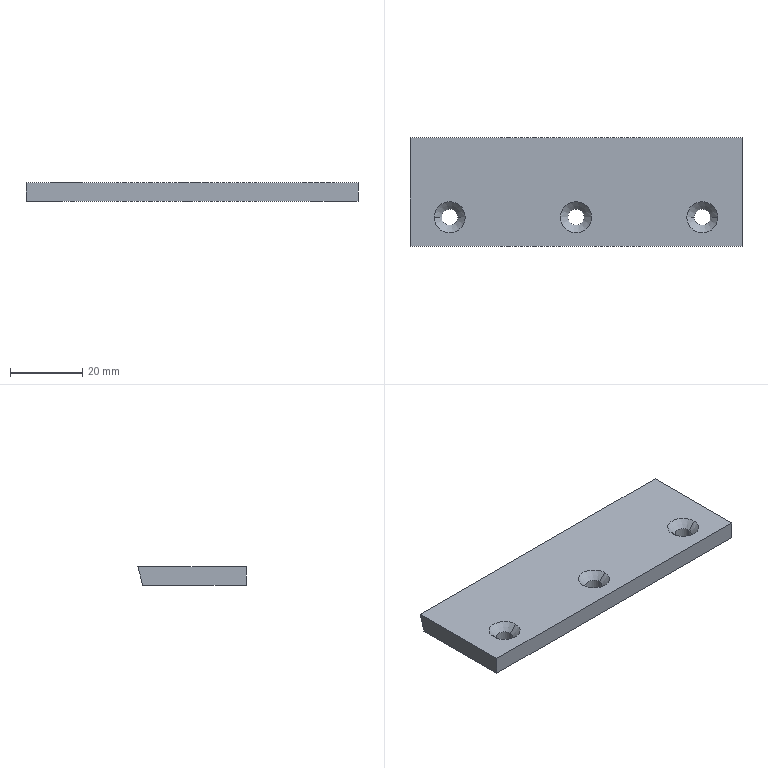Part | STEP file | 2030 Blade A | 1 solid | 18 faces | box 92 x 30 x 5 mm | volume 13137 mm3 | cone 6 | cylinder 6 | plane 6 | commonest cylinder face diameters 4.5 x6
STEP:
#1=CARTESIAN_POINT('',(0.,0.,0.));
#2=DIRECTION('',(0.,0.,1.));
#3=DIRECTION('',(1.,0.,0.));
#4=AXIS2_PLACEMENT_3D('',#1,#2,#3);
#5=CARTESIAN_POINT('',(-32.75,-7.,2.95));
#6=VERTEX_POINT('',#5);
#7=CARTESIAN_POINT('',(-30.7,-7.,5.));
#8=VERTEX_POINT('',#7);
#9=CARTESIAN_POINT('',(-30.7,-7.,5.));
#10=DIRECTION('',(0.7071,0.,0.7071));
#11=VECTOR('',#10,1.);
#12=LINE('',#9,#11);
#13=CARTESIAN_POINT('',(-35.,-7.,5.));
#14=DIRECTION('',(0.,0.,1.));
#15=DIRECTION('',(1.,0.,0.));
#16=AXIS2_PLACEMENT_3D('',#13,#14,#15);
#17=CONICAL_SURFACE('',#16,4.3,0.7854);
#18=CARTESIAN_POINT('',(6.283,0.));
#19=DIRECTION('',(0.,1.));
#20=VECTOR('',#19,1.);
#21=LINE('',#18,#20);
#22=(GEOMETRIC_REPRESENTATION_CONTEXT(2)PARAMETRIC_REPRESENTATION_CONTEXT()REPRESENTATION_CONTEXT('',''));
#23=DEFINITIONAL_REPRESENTATION('',(#21),#22);
#24=PCURVE('',#17,#23);
#25=CARTESIAN_POINT('',(-35.,-7.,5.));
#26=DIRECTION('',(0.,0.,1.));
#27=DIRECTION('',(1.,0.,0.));
#28=AXIS2_PLACEMENT_3D('',#25,#26,#27);
#29=CONICAL_SURFACE('',#28,4.3,0.7854);
#30=CARTESIAN_POINT('',(0.,0.));
#31=DIRECTION('',(0.,1.));
#32=VECTOR('',#31,1.);
#33=LINE('',#30,#32);
#34=(GEOMETRIC_REPRESENTATION_CONTEXT(2)PARAMETRIC_REPRESENTATION_CONTEXT()REPRESENTATION_CONTEXT('',''));
#35=DEFINITIONAL_REPRESENTATION('',(#33),#34);
#36=PCURVE('',#29,#35);
#37=SURFACE_CURVE('',#12,(#24,#36),.PCURVE_S1.);
#38=EDGE_CURVE('',#6,#8,#37,.T.);
#39=ORIENTED_EDGE('',*,*,#38,.T.);
#40=CARTESIAN_POINT('',(-39.3,-7.,5.));
#41=VERTEX_POINT('',#40);
#42=CARTESIAN_POINT('',(-35.,-7.,5.));
#43=DIRECTION('',(0.,0.,1.));
#44=DIRECTION('',(1.,0.,0.));
#45=AXIS2_PLACEMENT_3D('',#42,#43,#44);
#46=CIRCLE('',#45,4.3);
#47=CARTESIAN_POINT('',(0.,0.));
#48=DIRECTION('',(1.,0.));
#49=VECTOR('',#48,1.);
#50=LINE('',#47,#49);
#51=(GEOMETRIC_REPRESENTATION_CONTEXT(2)PARAMETRIC_REPRESENTATION_CONTEXT()REPRESENTATION_CONTEXT('',''));
#52=DEFINITIONAL_REPRESENTATION('',(#50),#51);
#53=PCURVE('',#17,#52);
#54=CARTESIAN_POINT('',(0.,0.,5.));
#55=DIRECTION('',(0.,0.,-1.));
#56=DIRECTION('',(-1.,0.,0.));
#57=AXIS2_PLACEMENT_3D('',#54,#55,#56);
#58=PLANE('',#57);
#59=CARTESIAN_POINT('',(30.7,-7.));
#60=CARTESIAN_POINT('',(30.7,0.4478));
#61=CARTESIAN_POINT('',(37.15,-3.276));
#62=CARTESIAN_POINT('',(43.6,-7.));
#63=CARTESIAN_POINT('',(37.15,-10.724));
#64=CARTESIAN_POINT('',(30.7,-14.448));
#65=CARTESIAN_POINT('',(30.7,-7.));
#66=(BOUNDED_CURVE()B_SPLINE_CURVE(2,(#59,#60,#61,#62,#63,#64,#65),.UNSPECIFIED.,.T.,.F.)B_SPLINE_CURVE_WITH_KNOTS((1,2,2,2,2,1),(-2.094,0.,2.094,4.189,6.283,8.378),.UNSPECIFIED.)CURVE()GEOMETRIC_REPRESENTATION_ITEM()RATIONAL_B_SPLINE_CURVE((1.,0.5,1.,0.5,1.,0.5,1.))REPRESENTATION_ITEM(''));
#67=(GEOMETRIC_REPRESENTATION_CONTEXT(2)PARAMETRIC_REPRESENTATION_CONTEXT()REPRESENTATION_CONTEXT('',''));
#68=DEFINITIONAL_REPRESENTATION('',(#66),#67);
#69=PCURVE('',#58,#68);
#70=SURFACE_CURVE('',#46,(#53,#69),.PCURVE_S1.);
#71=EDGE_CURVE('',#41,#8,#70,.T.);
#72=ORIENTED_EDGE('',*,*,#71,.F.);
#73=CARTESIAN_POINT('',(-37.25,-7.,2.95));
#74=VERTEX_POINT('',#73);
#75=CARTESIAN_POINT('',(-39.3,-7.,5.));
#76=DIRECTION('',(-0.7071,0.,0.7071));
#77=VECTOR('',#76,1.);
#78=LINE('',#75,#77);
#79=CARTESIAN_POINT('',(3.142,0.));
#80=DIRECTION('',(0.,1.));
#81=VECTOR('',#80,1.);
#82=LINE('',#79,#81);
#83=(GEOMETRIC_REPRESENTATION_CONTEXT(2)PARAMETRIC_REPRESENTATION_CONTEXT()REPRESENTATION_CONTEXT('',''));
#84=DEFINITIONAL_REPRESENTATION('',(#82),#83);
#85=PCURVE('',#17,#84);
#86=CARTESIAN_POINT('',(3.142,0.));
#87=DIRECTION('',(0.,1.));
#88=VECTOR('',#87,1.);
#89=LINE('',#86,#88);
#90=(GEOMETRIC_REPRESENTATION_CONTEXT(2)PARAMETRIC_REPRESENTATION_CONTEXT()REPRESENTATION_CONTEXT('',''));
#91=DEFINITIONAL_REPRESENTATION('',(#89),#90);
#92=PCURVE('',#29,#91);
#93=SURFACE_CURVE('',#78,(#85,#92),.PCURVE_S1.);
#94=EDGE_CURVE('',#74,#41,#93,.T.);
#95=ORIENTED_EDGE('',*,*,#94,.F.);
#96=CARTESIAN_POINT('',(-35.,-7.,2.95));
#97=DIRECTION('',(0.,0.,1.));
#98=DIRECTION('',(1.,0.,0.));
#99=AXIS2_PLACEMENT_3D('',#96,#97,#98);
#100=CIRCLE('',#99,2.25);
#101=CARTESIAN_POINT('',(0.,-2.05));
#102=DIRECTION('',(1.,0.));
#103=VECTOR('',#102,1.);
#104=LINE('',#101,#103);
#105=(GEOMETRIC_REPRESENTATION_CONTEXT(2)PARAMETRIC_REPRESENTATION_CONTEXT()REPRESENTATION_CONTEXT('',''));
#106=DEFINITIONAL_REPRESENTATION('',(#104),#105);
#107=PCURVE('',#17,#106);
#108=CARTESIAN_POINT('',(-35.,-7.,5.));
#109=DIRECTION('',(0.,0.,1.));
#110=DIRECTION('',(1.,0.,0.));
#111=AXIS2_PLACEMENT_3D('',#108,#109,#110);
#112=CYLINDRICAL_SURFACE('',#111,2.25);
#113=CARTESIAN_POINT('',(0.,-2.05));
#114=DIRECTION('',(1.,0.));
#115=VECTOR('',#114,1.);
#116=LINE('',#113,#115);
#117=(GEOMETRIC_REPRESENTATION_CONTEXT(2)PARAMETRIC_REPRESENTATION_CONTEXT()REPRESENTATION_CONTEXT('',''));
#118=DEFINITIONAL_REPRESENTATION('',(#116),#117);
#119=PCURVE('',#112,#118);
#120=SURFACE_CURVE('',#100,(#107,#119),.PCURVE_S1.);
#121=EDGE_CURVE('',#74,#6,#120,.T.);
#122=ORIENTED_EDGE('',*,*,#121,.T.);
#123=EDGE_LOOP('',(#39,#72,#95,#122));
#124=FACE_BOUND('',#123,.F.);
#125=ADVANCED_FACE('',(#124),#17,.F.);
#126=CARTESIAN_POINT('',(-32.75,-7.,0.));
#127=VERTEX_POINT('',#126);
#128=CARTESIAN_POINT('',(-32.75,-7.,5.));
#129=DIRECTION('',(0.,0.,1.));
#130=VECTOR('',#129,1.);
#131=LINE('',#128,#130);
#132=CARTESIAN_POINT('',(6.283,0.));
#133=DIRECTION('',(0.,1.));
#134=VECTOR('',#133,1.);
#135=LINE('',#132,#134);
#136=(GEOMETRIC_REPRESENTATION_CONTEXT(2)PARAMETRIC_REPRESENTATION_CONTEXT()REPRESENTATION_CONTEXT('',''));
#137=DEFINITIONAL_REPRESENTATION('',(#135),#136);
#138=PCURVE('',#112,#137);
#139=CARTESIAN_POINT('',(-35.,-7.,5.));
#140=DIRECTION('',(0.,0.,1.));
#141=DIRECTION('',(1.,0.,0.));
#142=AXIS2_PLACEMENT_3D('',#139,#140,#141);
#143=CYLINDRICAL_SURFACE('',#142,2.25);
#144=CARTESIAN_POINT('',(0.,0.));
#145=DIRECTION('',(0.,1.));
#146=VECTOR('',#145,1.);
#147=LINE('',#144,#146);
#148=(GEOMETRIC_REPRESENTATION_CONTEXT(2)PARAMETRIC_REPRESENTATION_CONTEXT()REPRESENTATION_CONTEXT('',''));
#149=DEFINITIONAL_REPRESENTATION('',(#147),#148);
#150=PCURVE('',#143,#149);
#151=SURFACE_CURVE('',#131,(#138,#150),.PCURVE_S1.);
#152=EDGE_CURVE('',#127,#6,#151,.T.);
#153=ORIENTED_EDGE('',*,*,#152,.T.);
#154=ORIENTED_EDGE('',*,*,#121,.F.);
#155=CARTESIAN_POINT('',(-37.25,-7.,0.));
#156=VERTEX_POINT('',#155);
#157=CARTESIAN_POINT('',(-37.25,-7.,5.));
#158=DIRECTION('',(0.,0.,1.));
#159=VECTOR('',#158,1.);
#160=LINE('',#157,#159);
#161=CARTESIAN_POINT('',(3.142,0.));
#162=DIRECTION('',(0.,1.));
#163=VECTOR('',#162,1.);
#164=LINE('',#161,#163);
#165=(GEOMETRIC_REPRESENTATION_CONTEXT(2)PARAMETRIC_REPRESENTATION_CONTEXT()REPRESENTATION_CONTEXT('',''));
#166=DEFINITIONAL_REPRESENTATION('',(#164),#165);
#167=PCURVE('',#112,#166);
#168=CARTESIAN_POINT('',(3.142,0.));
#169=DIRECTION('',(0.,1.));
#170=VECTOR('',#169,1.);
#171=LINE('',#168,#170);
#172=(GEOMETRIC_REPRESENTATION_CONTEXT(2)PARAMETRIC_REPRESENTATION_CONTEXT()REPRESENTATION_CONTEXT('',''));
#173=DEFINITIONAL_REPRESENTATION('',(#171),#172);
#174=PCURVE('',#143,#173);
#175=SURFACE_CURVE('',#160,(#167,#174),.PCURVE_S1.);
#176=EDGE_CURVE('',#156,#74,#175,.T.);
#177=ORIENTED_EDGE('',*,*,#176,.F.);
#178=CARTESIAN_POINT('',(-35.,-7.,0.));
#179=DIRECTION('',(0.,0.,1.));
#180=DIRECTION('',(1.,0.,0.));
#181=AXIS2_PLACEMENT_3D('',#178,#179,#180);
#182=CIRCLE('',#181,2.25);
#183=CARTESIAN_POINT('',(0.,-5.));
#184=DIRECTION('',(1.,0.));
#185=VECTOR('',#184,1.);
#186=LINE('',#183,#185);
#187=(GEOMETRIC_REPRESENTATION_CONTEXT(2)PARAMETRIC_REPRESENTATION_CONTEXT()REPRESENTATION_CONTEXT('',''));
#188=DEFINITIONAL_REPRESENTATION('',(#186),#187);
#189=PCURVE('',#112,#188);
#190=CARTESIAN_POINT('',(0.,0.,0.));
#191=DIRECTION('',(0.,0.,-1.));
#192=DIRECTION('',(-1.,0.,0.));
#193=AXIS2_PLACEMENT_3D('',#190,#191,#192);
#194=PLANE('',#193);
#195=CARTESIAN_POINT('',(32.75,-7.));
#196=CARTESIAN_POINT('',(32.75,-3.103));
#197=CARTESIAN_POINT('',(36.125,-5.051));
#198=CARTESIAN_POINT('',(39.5,-7.));
#199=CARTESIAN_POINT('',(36.125,-8.949));
#200=CARTESIAN_POINT('',(32.75,-10.897));
#201=CARTESIAN_POINT('',(32.75,-7.));
#202=(BOUNDED_CURVE()B_SPLINE_CURVE(2,(#195,#196,#197,#198,#199,#200,#201),.UNSPECIFIED.,.T.,.F.)B_SPLINE_CURVE_WITH_KNOTS((1,2,2,2,2,1),(-2.094,0.,2.094,4.189,6.283,8.378),.UNSPECIFIED.)CURVE()GEOMETRIC_REPRESENTATION_ITEM()RATIONAL_B_SPLINE_CURVE((1.,0.5,1.,0.5,1.,0.5,1.))REPRESENTATION_ITEM(''));
#203=(GEOMETRIC_REPRESENTATION_CONTEXT(2)PARAMETRIC_REPRESENTATION_CONTEXT()REPRESENTATION_CONTEXT('',''));
#204=DEFINITIONAL_REPRESENTATION('',(#202),#203);
#205=PCURVE('',#194,#204);
#206=SURFACE_CURVE('',#182,(#189,#205),.PCURVE_S1.);
#207=EDGE_CURVE('',#156,#127,#206,.T.);
#208=ORIENTED_EDGE('',*,*,#207,.T.);
#209=EDGE_LOOP('',(#153,#154,#177,#208));
#210=FACE_BOUND('',#209,.F.);
#211=ADVANCED_FACE('',(#210),#112,.F.);
#212=CARTESIAN_POINT('',(2.25,-7.,2.95));
#213=VERTEX_POINT('',#212);
#214=CARTESIAN_POINT('',(4.3,-7.,5.));
#215=VERTEX_POINT('',#214);
#216=CARTESIAN_POINT('',(4.3,-7.,5.));
#217=DIRECTION('',(0.7071,0.,0.7071));
#218=VECTOR('',#217,1.);
#219=LINE('',#216,#218);
#220=CARTESIAN_POINT('',(0.,-7.,5.));
#221=DIRECTION('',(0.,0.,1.));
#222=DIRECTION('',(1.,0.,0.));
#223=AXIS2_PLACEMENT_3D('',#220,#221,#222);
#224=CONICAL_SURFACE('',#223,4.3,0.7854);
#225=CARTESIAN_POINT('',(6.283,0.));
#226=DIRECTION('',(0.,1.));
#227=VECTOR('',#226,1.);
#228=LINE('',#225,#227);
#229=(GEOMETRIC_REPRESENTATION_CONTEXT(2)PARAMETRIC_REPRESENTATION_CONTEXT()REPRESENTATION_CONTEXT('',''));
#230=DEFINITIONAL_REPRESENTATION('',(#228),#229);
#231=PCURVE('',#224,#230);
#232=CARTESIAN_POINT('',(0.,-7.,5.));
#233=DIRECTION('',(0.,0.,1.));
#234=DIRECTION('',(1.,0.,0.));
#235=AXIS2_PLACEMENT_3D('',#232,#233,#234);
#236=CONICAL_SURFACE('',#235,4.3,0.7854);
#237=CARTESIAN_POINT('',(0.,0.));
#238=DIRECTION('',(0.,1.));
#239=VECTOR('',#238,1.);
#240=LINE('',#237,#239);
#241=(GEOMETRIC_REPRESENTATION_CONTEXT(2)PARAMETRIC_REPRESENTATION_CONTEXT()REPRESENTATION_CONTEXT('',''));
#242=DEFINITIONAL_REPRESENTATION('',(#240),#241);
#243=PCURVE('',#236,#242);
#244=SURFACE_CURVE('',#219,(#231,#243),.PCURVE_S1.);
#245=EDGE_CURVE('',#213,#215,#244,.T.);
#246=ORIENTED_EDGE('',*,*,#245,.T.);
#247=CARTESIAN_POINT('',(-4.3,-7.,5.));
#248=VERTEX_POINT('',#247);
#249=CARTESIAN_POINT('',(0.,-7.,5.));
#250=DIRECTION('',(0.,0.,1.));
#251=DIRECTION('',(1.,0.,0.));
#252=AXIS2_PLACEMENT_3D('',#249,#250,#251);
#253=CIRCLE('',#252,4.3);
#254=CARTESIAN_POINT('',(0.,0.));
#255=DIRECTION('',(1.,0.));
#256=VECTOR('',#255,1.);
#257=LINE('',#254,#256);
#258=(GEOMETRIC_REPRESENTATION_CONTEXT(2)PARAMETRIC_REPRESENTATION_CONTEXT()REPRESENTATION_CONTEXT('',''));
#259=DEFINITIONAL_REPRESENTATION('',(#257),#258);
#260=PCURVE('',#224,#259);
#261=CARTESIAN_POINT('',(-4.3,-7.));
#262=CARTESIAN_POINT('',(-4.3,0.4478));
#263=CARTESIAN_POINT('',(2.15,-3.276));
#264=CARTESIAN_POINT('',(8.6,-7.));
#265=CARTESIAN_POINT('',(2.15,-10.724));
#266=CARTESIAN_POINT('',(-4.3,-14.448));
#267=CARTESIAN_POINT('',(-4.3,-7.));
#268=(BOUNDED_CURVE()B_SPLINE_CURVE(2,(#261,#262,#263,#264,#265,#266,#267),.UNSPECIFIED.,.T.,.F.)B_SPLINE_CURVE_WITH_KNOTS((1,2,2,2,2,1),(-2.094,0.,2.094,4.189,6.283,8.378),.UNSPECIFIED.)CURVE()GEOMETRIC_REPRESENTATION_ITEM()RATIONAL_B_SPLINE_CURVE((1.,0.5,1.,0.5,1.,0.5,1.))REPRESENTATION_ITEM(''));
#269=(GEOMETRIC_REPRESENTATION_CONTEXT(2)PARAMETRIC_REPRESENTATION_CONTEXT()REPRESENTATION_CONTEXT('',''));
#270=DEFINITIONAL_REPRESENTATION('',(#268),#269);
#271=PCURVE('',#58,#270);
#272=SURFACE_CURVE('',#253,(#260,#271),.PCURVE_S1.);
#273=EDGE_CURVE('',#248,#215,#272,.T.);
#274=ORIENTED_EDGE('',*,*,#273,.F.);
#275=CARTESIAN_POINT('',(-2.25,-7.,2.95));
#276=VERTEX_POINT('',#275);
#277=CARTESIAN_POINT('',(-4.3,-7.,5.));
#278=DIRECTION('',(-0.7071,0.,0.7071));
#279=VECTOR('',#278,1.);
#280=LINE('',#277,#279);
#281=CARTESIAN_POINT('',(3.142,0.));
#282=DIRECTION('',(0.,1.));
#283=VECTOR('',#282,1.);
#284=LINE('',#281,#283);
#285=(GEOMETRIC_REPRESENTATION_CONTEXT(2)PARAMETRIC_REPRESENTATION_CONTEXT()REPRESENTATION_CONTEXT('',''));
#286=DEFINITIONAL_REPRESENTATION('',(#284),#285);
#287=PCURVE('',#224,#286);
#288=CARTESIAN_POINT('',(3.142,0.));
#289=DIRECTION('',(0.,1.));
#290=VECTOR('',#289,1.);
#291=LINE('',#288,#290);
#292=(GEOMETRIC_REPRESENTATION_CONTEXT(2)PARAMETRIC_REPRESENTATION_CONTEXT()REPRESENTATION_CONTEXT('',''));
#293=DEFINITIONAL_REPRESENTATION('',(#291),#292);
#294=PCURVE('',#236,#293);
#295=SURFACE_CURVE('',#280,(#287,#294),.PCURVE_S1.);
#296=EDGE_CURVE('',#276,#248,#295,.T.);
#297=ORIENTED_EDGE('',*,*,#296,.F.);
#298=CARTESIAN_POINT('',(0.,-7.,2.95));
#299=DIRECTION('',(0.,0.,1.));
#300=DIRECTION('',(1.,0.,0.));
#301=AXIS2_PLACEMENT_3D('',#298,#299,#300);
#302=CIRCLE('',#301,2.25);
#303=CARTESIAN_POINT('',(0.,-2.05));
#304=DIRECTION('',(1.,0.));
#305=VECTOR('',#304,1.);
#306=LINE('',#303,#305);
#307=(GEOMETRIC_REPRESENTATION_CONTEXT(2)PARAMETRIC_REPRESENTATION_CONTEXT()REPRESENTATION_CONTEXT('',''));
#308=DEFINITIONAL_REPRESENTATION('',(#306),#307);
#309=PCURVE('',#224,#308);
#310=CARTESIAN_POINT('',(0.,-7.,5.));
#311=DIRECTION('',(0.,0.,1.));
#312=DIRECTION('',(1.,0.,0.));
#313=AXIS2_PLACEMENT_3D('',#310,#311,#312);
#314=CYLINDRICAL_SURFACE('',#313,2.25);
#315=CARTESIAN_POINT('',(0.,-2.05));
#316=DIRECTION('',(1.,0.));
#317=VECTOR('',#316,1.);
#318=LINE('',#315,#317);
#319=(GEOMETRIC_REPRESENTATION_CONTEXT(2)PARAMETRIC_REPRESENTATION_CONTEXT()REPRESENTATION_CONTEXT('',''));
#320=DEFINITIONAL_REPRESENTATION('',(#318),#319);
#321=PCURVE('',#314,#320);
#322=SURFACE_CURVE('',#302,(#309,#321),.PCURVE_S1.);
#323=EDGE_CURVE('',#276,#213,#322,.T.);
#324=ORIENTED_EDGE('',*,*,#323,.T.);
#325=EDGE_LOOP('',(#246,#274,#297,#324));
#326=FACE_BOUND('',#325,.F.);
#327=ADVANCED_FACE('',(#326),#224,.F.);
#328=CARTESIAN_POINT('',(2.25,-7.,0.));
#329=VERTEX_POINT('',#328);
#330=CARTESIAN_POINT('',(2.25,-7.,5.));
#331=DIRECTION('',(0.,0.,1.));
#332=VECTOR('',#331,1.);
#333=LINE('',#330,#332);
#334=CARTESIAN_POINT('',(6.283,0.));
#335=DIRECTION('',(0.,1.));
#336=VECTOR('',#335,1.);
#337=LINE('',#334,#336);
#338=(GEOMETRIC_REPRESENTATION_CONTEXT(2)PARAMETRIC_REPRESENTATION_CONTEXT()REPRESENTATION_CONTEXT('',''));
#339=DEFINITIONAL_REPRESENTATION('',(#337),#338);
#340=PCURVE('',#314,#339);
#341=CARTESIAN_POINT('',(0.,-7.,5.));
#342=DIRECTION('',(0.,0.,1.));
#343=DIRECTION('',(1.,0.,0.));
#344=AXIS2_PLACEMENT_3D('',#341,#342,#343);
#345=CYLINDRICAL_SURFACE('',#344,2.25);
#346=CARTESIAN_POINT('',(0.,0.));
#347=DIRECTION('',(0.,1.));
#348=VECTOR('',#347,1.);
#349=LINE('',#346,#348);
#350=(GEOMETRIC_REPRESENTATION_CONTEXT(2)PARAMETRIC_REPRESENTATION_CONTEXT()REPRESENTATION_CONTEXT('',''));
#351=DEFINITIONAL_REPRESENTATION('',(#349),#350);
#352=PCURVE('',#345,#351);
#353=SURFACE_CURVE('',#333,(#340,#352),.PCURVE_S1.);
#354=EDGE_CURVE('',#329,#213,#353,.T.);
#355=ORIENTED_EDGE('',*,*,#354,.T.);
#356=ORIENTED_EDGE('',*,*,#323,.F.);
#357=CARTESIAN_POINT('',(-2.25,-7.,0.));
#358=VERTEX_POINT('',#357);
#359=CARTESIAN_POINT('',(-2.25,-7.,5.));
#360=DIRECTION('',(0.,0.,1.));
#361=VECTOR('',#360,1.);
#362=LINE('',#359,#361);
#363=CARTESIAN_POINT('',(3.142,0.));
#364=DIRECTION('',(0.,1.));
#365=VECTOR('',#364,1.);
#366=LINE('',#363,#365);
#367=(GEOMETRIC_REPRESENTATION_CONTEXT(2)PARAMETRIC_REPRESENTATION_CONTEXT()REPRESENTATION_CONTEXT('',''));
#368=DEFINITIONAL_REPRESENTATION('',(#366),#367);
#369=PCURVE('',#314,#368);
#370=CARTESIAN_POINT('',(3.142,0.));
#371=DIRECTION('',(0.,1.));
#372=VECTOR('',#371,1.);
#373=LINE('',#370,#372);
#374=(GEOMETRIC_REPRESENTATION_CONTEXT(2)PARAMETRIC_REPRESENTATION_CONTEXT()REPRESENTATION_CONTEXT('',''));
#375=DEFINITIONAL_REPRESENTATION('',(#373),#374);
#376=PCURVE('',#345,#375);
#377=SURFACE_CURVE('',#362,(#369,#376),.PCURVE_S1.);
#378=EDGE_CURVE('',#358,#276,#377,.T.);
#379=ORIENTED_EDGE('',*,*,#378,.F.);
#380=CARTESIAN_POINT('',(0.,-7.,0.));
#381=DIRECTION('',(0.,0.,1.));
#382=DIRECTION('',(1.,0.,0.));
#383=AXIS2_PLACEMENT_3D('',#380,#381,#382);
#384=CIRCLE('',#383,2.25);
#385=CARTESIAN_POINT('',(0.,-5.));
#386=DIRECTION('',(1.,0.));
#387=VECTOR('',#386,1.);
#388=LINE('',#385,#387);
#389=(GEOMETRIC_REPRESENTATION_CONTEXT(2)PARAMETRIC_REPRESENTATION_CONTEXT()REPRESENTATION_CONTEXT('',''));
#390=DEFINITIONAL_REPRESENTATION('',(#388),#389);
#391=PCURVE('',#314,#390);
#392=CARTESIAN_POINT('',(-2.25,-7.));
#393=CARTESIAN_POINT('',(-2.25,-3.103));
#394=CARTESIAN_POINT('',(1.125,-5.051));
#395=CARTESIAN_POINT('',(4.5,-7.));
#396=CARTESIAN_POINT('',(1.125,-8.949));
#397=CARTESIAN_POINT('',(-2.25,-10.897));
#398=CARTESIAN_POINT('',(-2.25,-7.));
#399=(BOUNDED_CURVE()B_SPLINE_CURVE(2,(#392,#393,#394,#395,#396,#397,#398),.UNSPECIFIED.,.T.,.F.)B_SPLINE_CURVE_WITH_KNOTS((1,2,2,2,2,1),(-2.094,0.,2.094,4.189,6.283,8.378),.UNSPECIFIED.)CURVE()GEOMETRIC_REPRESENTATION_ITEM()RATIONAL_B_SPLINE_CURVE((1.,0.5,1.,0.5,1.,0.5,1.))REPRESENTATION_ITEM(''));
#400=(GEOMETRIC_REPRESENTATION_CONTEXT(2)PARAMETRIC_REPRESENTATION_CONTEXT()REPRESENTATION_CONTEXT('',''));
#401=DEFINITIONAL_REPRESENTATION('',(#399),#400);
#402=PCURVE('',#194,#401);
#403=SURFACE_CURVE('',#384,(#391,#402),.PCURVE_S1.);
#404=EDGE_CURVE('',#358,#329,#403,.T.);
#405=ORIENTED_EDGE('',*,*,#404,.T.);
#406=EDGE_LOOP('',(#355,#356,#379,#405));
#407=FACE_BOUND('',#406,.F.);
#408=ADVANCED_FACE('',(#407),#314,.F.);
#409=CARTESIAN_POINT('',(37.25,-7.,2.95));
#410=VERTEX_POINT('',#409);
#411=CARTESIAN_POINT('',(39.3,-7.,5.));
#412=VERTEX_POINT('',#411);
#413=CARTESIAN_POINT('',(39.3,-7.,5.));
#414=DIRECTION('',(0.7071,0.,0.7071));
#415=VECTOR('',#414,1.);
#416=LINE('',#413,#415);
#417=CARTESIAN_POINT('',(35.,-7.,5.));
#418=DIRECTION('',(0.,0.,1.));
#419=DIRECTION('',(1.,0.,0.));
#420=AXIS2_PLACEMENT_3D('',#417,#418,#419);
#421=CONICAL_SURFACE('',#420,4.3,0.7854);
#422=CARTESIAN_POINT('',(6.283,0.));
#423=DIRECTION('',(0.,1.));
#424=VECTOR('',#423,1.);
#425=LINE('',#422,#424);
#426=(GEOMETRIC_REPRESENTATION_CONTEXT(2)PARAMETRIC_REPRESENTATION_CONTEXT()REPRESENTATION_CONTEXT('',''));
#427=DEFINITIONAL_REPRESENTATION('',(#425),#426);
#428=PCURVE('',#421,#427);
#429=CARTESIAN_POINT('',(35.,-7.,5.));
#430=DIRECTION('',(0.,0.,1.));
#431=DIRECTION('',(1.,0.,0.));
#432=AXIS2_PLACEMENT_3D('',#429,#430,#431);
#433=CONICAL_SURFACE('',#432,4.3,0.7854);
#434=CARTESIAN_POINT('',(0.,0.));
#435=DIRECTION('',(0.,1.));
#436=VECTOR('',#435,1.);
#437=LINE('',#434,#436);
#438=(GEOMETRIC_REPRESENTATION_CONTEXT(2)PARAMETRIC_REPRESENTATION_CONTEXT()REPRESENTATION_CONTEXT('',''));
#439=DEFINITIONAL_REPRESENTATION('',(#437),#438);
#440=PCURVE('',#433,#439);
#441=SURFACE_CURVE('',#416,(#428,#440),.PCURVE_S1.);
#442=EDGE_CURVE('',#410,#412,#441,.T.);
#443=ORIENTED_EDGE('',*,*,#442,.T.);
#444=CARTESIAN_POINT('',(30.7,-7.,5.));
#445=VERTEX_POINT('',#444);
#446=CARTESIAN_POINT('',(35.,-7.,5.));
#447=DIRECTION('',(0.,0.,1.));
#448=DIRECTION('',(1.,0.,0.));
#449=AXIS2_PLACEMENT_3D('',#446,#447,#448);
#450=CIRCLE('',#449,4.3);
#451=CARTESIAN_POINT('',(0.,0.));
#452=DIRECTION('',(1.,0.));
#453=VECTOR('',#452,1.);
#454=LINE('',#451,#453);
#455=(GEOMETRIC_REPRESENTATION_CONTEXT(2)PARAMETRIC_REPRESENTATION_CONTEXT()REPRESENTATION_CONTEXT('',''));
#456=DEFINITIONAL_REPRESENTATION('',(#454),#455);
#457=PCURVE('',#421,#456);
#458=CARTESIAN_POINT('',(-39.3,-7.));
#459=CARTESIAN_POINT('',(-39.3,0.4478));
#460=CARTESIAN_POINT('',(-32.85,-3.276));
#461=CARTESIAN_POINT('',(-26.4,-7.));
#462=CARTESIAN_POINT('',(-32.85,-10.724));
#463=CARTESIAN_POINT('',(-39.3,-14.448));
#464=CARTESIAN_POINT('',(-39.3,-7.));
#465=(BOUNDED_CURVE()B_SPLINE_CURVE(2,(#458,#459,#460,#461,#462,#463,#464),.UNSPECIFIED.,.T.,.F.)B_SPLINE_CURVE_WITH_KNOTS((1,2,2,2,2,1),(-2.094,0.,2.094,4.189,6.283,8.378),.UNSPECIFIED.)CURVE()GEOMETRIC_REPRESENTATION_ITEM()RATIONAL_B_SPLINE_CURVE((1.,0.5,1.,0.5,1.,0.5,1.))REPRESENTATION_ITEM(''));
#466=(GEOMETRIC_REPRESENTATION_CONTEXT(2)PARAMETRIC_REPRESENTATION_CONTEXT()REPRESENTATION_CONTEXT('',''));
#467=DEFINITIONAL_REPRESENTATION('',(#465),#466);
#468=PCURVE('',#58,#467);
#469=SURFACE_CURVE('',#450,(#457,#468),.PCURVE_S1.);
#470=EDGE_CURVE('',#445,#412,#469,.T.);
#471=ORIENTED_EDGE('',*,*,#470,.F.);
#472=CARTESIAN_POINT('',(32.75,-7.,2.95));
#473=VERTEX_POINT('',#472);
#474=CARTESIAN_POINT('',(30.7,-7.,5.));
#475=DIRECTION('',(-0.7071,0.,0.7071));
#476=VECTOR('',#475,1.);
#477=LINE('',#474,#476);
#478=CARTESIAN_POINT('',(3.142,0.));
#479=DIRECTION('',(0.,1.));
#480=VECTOR('',#479,1.);
#481=LINE('',#478,#480);
#482=(GEOMETRIC_REPRESENTATION_CONTEXT(2)PARAMETRIC_REPRESENTATION_CONTEXT()REPRESENTATION_CONTEXT('',''));
#483=DEFINITIONAL_REPRESENTATION('',(#481),#482);
#484=PCURVE('',#421,#483);
#485=CARTESIAN_POINT('',(3.142,0.));
#486=DIRECTION('',(0.,1.));
#487=VECTOR('',#486,1.);
#488=LINE('',#485,#487);
#489=(GEOMETRIC_REPRESENTATION_CONTEXT(2)PARAMETRIC_REPRESENTATION_CONTEXT()REPRESENTATION_CONTEXT('',''));
#490=DEFINITIONAL_REPRESENTATION('',(#488),#489);
#491=PCURVE('',#433,#490);
#492=SURFACE_CURVE('',#477,(#484,#491),.PCURVE_S1.);
#493=EDGE_CURVE('',#473,#445,#492,.T.);
#494=ORIENTED_EDGE('',*,*,#493,.F.);
#495=CARTESIAN_POINT('',(35.,-7.,2.95));
#496=DIRECTION('',(0.,0.,1.));
#497=DIRECTION('',(1.,0.,0.));
#498=AXIS2_PLACEMENT_3D('',#495,#496,#497);
#499=CIRCLE('',#498,2.25);
#500=CARTESIAN_POINT('',(0.,-2.05));
#501=DIRECTION('',(1.,0.));
#502=VECTOR('',#501,1.);
#503=LINE('',#500,#502);
#504=(GEOMETRIC_REPRESENTATION_CONTEXT(2)PARAMETRIC_REPRESENTATION_CONTEXT()REPRESENTATION_CONTEXT('',''));
#505=DEFINITIONAL_REPRESENTATION('',(#503),#504);
#506=PCURVE('',#421,#505);
#507=CARTESIAN_POINT('',(35.,-7.,5.));
#508=DIRECTION('',(0.,0.,1.));
#509=DIRECTION('',(1.,0.,0.));
#510=AXIS2_PLACEMENT_3D('',#507,#508,#509);
#511=CYLINDRICAL_SURFACE('',#510,2.25);
#512=CARTESIAN_POINT('',(0.,-2.05));
#513=DIRECTION('',(1.,0.));
#514=VECTOR('',#513,1.);
#515=LINE('',#512,#514);
#516=(GEOMETRIC_REPRESENTATION_CONTEXT(2)PARAMETRIC_REPRESENTATION_CONTEXT()REPRESENTATION_CONTEXT('',''));
#517=DEFINITIONAL_REPRESENTATION('',(#515),#516);
#518=PCURVE('',#511,#517);
#519=SURFACE_CURVE('',#499,(#506,#518),.PCURVE_S1.);
#520=EDGE_CURVE('',#473,#410,#519,.T.);
#521=ORIENTED_EDGE('',*,*,#520,.T.);
#522=EDGE_LOOP('',(#443,#471,#494,#521));
#523=FACE_BOUND('',#522,.F.);
#524=ADVANCED_FACE('',(#523),#421,.F.);
#525=CARTESIAN_POINT('',(37.25,-7.,0.));
#526=VERTEX_POINT('',#525);
#527=CARTESIAN_POINT('',(37.25,-7.,5.));
#528=DIRECTION('',(0.,0.,1.));
#529=VECTOR('',#528,1.);
#530=LINE('',#527,#529);
#531=CARTESIAN_POINT('',(6.283,0.));
#532=DIRECTION('',(0.,1.));
#533=VECTOR('',#532,1.);
#534=LINE('',#531,#533);
#535=(GEOMETRIC_REPRESENTATION_CONTEXT(2)PARAMETRIC_REPRESENTATION_CONTEXT()REPRESENTATION_CONTEXT('',''));
#536=DEFINITIONAL_REPRESENTATION('',(#534),#535);
#537=PCURVE('',#511,#536);
#538=CARTESIAN_POINT('',(35.,-7.,5.));
#539=DIRECTION('',(0.,0.,1.));
#540=DIRECTION('',(1.,0.,0.));
#541=AXIS2_PLACEMENT_3D('',#538,#539,#540);
#542=CYLINDRICAL_SURFACE('',#541,2.25);
#543=CARTESIAN_POINT('',(0.,0.));
#544=DIRECTION('',(0.,1.));
#545=VECTOR('',#544,1.);
#546=LINE('',#543,#545);
#547=(GEOMETRIC_REPRESENTATION_CONTEXT(2)PARAMETRIC_REPRESENTATION_CONTEXT()REPRESENTATION_CONTEXT('',''));
#548=DEFINITIONAL_REPRESENTATION('',(#546),#547);
#549=PCURVE('',#542,#548);
#550=SURFACE_CURVE('',#530,(#537,#549),.PCURVE_S1.);
#551=EDGE_CURVE('',#526,#410,#550,.T.);
#552=ORIENTED_EDGE('',*,*,#551,.T.);
#553=ORIENTED_EDGE('',*,*,#520,.F.);
#554=CARTESIAN_POINT('',(32.75,-7.,0.));
#555=VERTEX_POINT('',#554);
#556=CARTESIAN_POINT('',(32.75,-7.,5.));
#557=DIRECTION('',(0.,0.,1.));
#558=VECTOR('',#557,1.);
#559=LINE('',#556,#558);
#560=CARTESIAN_POINT('',(3.142,0.));
#561=DIRECTION('',(0.,1.));
#562=VECTOR('',#561,1.);
#563=LINE('',#560,#562);
#564=(GEOMETRIC_REPRESENTATION_CONTEXT(2)PARAMETRIC_REPRESENTATION_CONTEXT()REPRESENTATION_CONTEXT('',''));
#565=DEFINITIONAL_REPRESENTATION('',(#563),#564);
#566=PCURVE('',#511,#565);
#567=CARTESIAN_POINT('',(3.142,0.));
#568=DIRECTION('',(0.,1.));
#569=VECTOR('',#568,1.);
#570=LINE('',#567,#569);
#571=(GEOMETRIC_REPRESENTATION_CONTEXT(2)PARAMETRIC_REPRESENTATION_CONTEXT()REPRESENTATION_CONTEXT('',''));
#572=DEFINITIONAL_REPRESENTATION('',(#570),#571);
#573=PCURVE('',#542,#572);
#574=SURFACE_CURVE('',#559,(#566,#573),.PCURVE_S1.);
#575=EDGE_CURVE('',#555,#473,#574,.T.);
#576=ORIENTED_EDGE('',*,*,#575,.F.);
#577=CARTESIAN_POINT('',(35.,-7.,0.));
#578=DIRECTION('',(0.,0.,1.));
#579=DIRECTION('',(1.,0.,0.));
#580=AXIS2_PLACEMENT_3D('',#577,#578,#579);
#581=CIRCLE('',#580,2.25);
#582=CARTESIAN_POINT('',(0.,-5.));
#583=DIRECTION('',(1.,0.));
#584=VECTOR('',#583,1.);
#585=LINE('',#582,#584);
#586=(GEOMETRIC_REPRESENTATION_CONTEXT(2)PARAMETRIC_REPRESENTATION_CONTEXT()REPRESENTATION_CONTEXT('',''));
#587=DEFINITIONAL_REPRESENTATION('',(#585),#586);
#588=PCURVE('',#511,#587);
#589=CARTESIAN_POINT('',(-37.25,-7.));
#590=CARTESIAN_POINT('',(-37.25,-3.103));
#591=CARTESIAN_POINT('',(-33.875,-5.051));
#592=CARTESIAN_POINT('',(-30.5,-7.));
#593=CARTESIAN_POINT('',(-33.875,-8.949));
#594=CARTESIAN_POINT('',(-37.25,-10.897));
#595=CARTESIAN_POINT('',(-37.25,-7.));
#596=(BOUNDED_CURVE()B_SPLINE_CURVE(2,(#589,#590,#591,#592,#593,#594,#595),.UNSPECIFIED.,.T.,.F.)B_SPLINE_CURVE_WITH_KNOTS((1,2,2,2,2,1),(-2.094,0.,2.094,4.189,6.283,8.378),.UNSPECIFIED.)CURVE()GEOMETRIC_REPRESENTATION_ITEM()RATIONAL_B_SPLINE_CURVE((1.,0.5,1.,0.5,1.,0.5,1.))REPRESENTATION_ITEM(''));
#597=(GEOMETRIC_REPRESENTATION_CONTEXT(2)PARAMETRIC_REPRESENTATION_CONTEXT()REPRESENTATION_CONTEXT('',''));
#598=DEFINITIONAL_REPRESENTATION('',(#596),#597);
#599=PCURVE('',#194,#598);
#600=SURFACE_CURVE('',#581,(#588,#599),.PCURVE_S1.);
#601=EDGE_CURVE('',#555,#526,#600,.T.);
#602=ORIENTED_EDGE('',*,*,#601,.T.);
#603=EDGE_LOOP('',(#552,#553,#576,#602));
#604=FACE_BOUND('',#603,.F.);
#605=ADVANCED_FACE('',(#604),#511,.F.);
#606=CARTESIAN_POINT('',(46.,-15.,0.));
#607=VERTEX_POINT('',#606);
#608=CARTESIAN_POINT('',(46.,13.66,0.));
#609=VERTEX_POINT('',#608);
#610=CARTESIAN_POINT('',(46.,-15.,0.));
#611=DIRECTION('',(0.,1.,0.));
#612=VECTOR('',#611,1.);
#613=LINE('',#610,#612);
#614=CARTESIAN_POINT('',(46.,-15.,5.));
#615=DIRECTION('',(-1.,0.,0.));
#616=DIRECTION('',(0.,0.,1.));
#617=AXIS2_PLACEMENT_3D('',#614,#615,#616);
#618=PLANE('',#617);
#619=CARTESIAN_POINT('',(-5.,0.));
#620=DIRECTION('',(0.,1.));
#621=VECTOR('',#620,1.);
#622=LINE('',#619,#621);
#623=(GEOMETRIC_REPRESENTATION_CONTEXT(2)PARAMETRIC_REPRESENTATION_CONTEXT()REPRESENTATION_CONTEXT('',''));
#624=DEFINITIONAL_REPRESENTATION('',(#622),#623);
#625=PCURVE('',#618,#624);
#626=CARTESIAN_POINT('',(-46.,-15.));
#627=DIRECTION('',(0.,1.));
#628=VECTOR('',#627,1.);
#629=LINE('',#626,#628);
#630=(GEOMETRIC_REPRESENTATION_CONTEXT(2)PARAMETRIC_REPRESENTATION_CONTEXT()REPRESENTATION_CONTEXT('',''));
#631=DEFINITIONAL_REPRESENTATION('',(#629),#630);
#632=PCURVE('',#194,#631);
#633=SURFACE_CURVE('',#613,(#625,#632),.PCURVE_S1.);
#634=EDGE_CURVE('',#607,#609,#633,.T.);
#635=ORIENTED_EDGE('',*,*,#634,.T.);
#636=CARTESIAN_POINT('',(46.,15.,5.));
#637=VERTEX_POINT('',#636);
#638=CARTESIAN_POINT('',(46.,15.,5.));
#639=DIRECTION('',(0.,-0.2588,-0.9659));
#640=VECTOR('',#639,1.);
#641=LINE('',#638,#640);
#642=CARTESIAN_POINT('',(0.,30.));
#643=DIRECTION('',(-0.9659,-0.2588));
#644=VECTOR('',#643,1.);
#645=LINE('',#642,#644);
#646=(GEOMETRIC_REPRESENTATION_CONTEXT(2)PARAMETRIC_REPRESENTATION_CONTEXT()REPRESENTATION_CONTEXT('',''));
#647=DEFINITIONAL_REPRESENTATION('',(#645),#646);
#648=PCURVE('',#618,#647);
#649=CARTESIAN_POINT('',(-46.,15.,5.));
#650=DIRECTION('',(0.,-0.9659,0.2588));
#651=DIRECTION('',(0.,-0.2588,-0.9659));
#652=AXIS2_PLACEMENT_3D('',#649,#650,#651);
#653=PLANE('',#652);
#654=CARTESIAN_POINT('',(0.,92.));
#655=DIRECTION('',(1.,0.));
#656=VECTOR('',#655,1.);
#657=LINE('',#654,#656);
#658=(GEOMETRIC_REPRESENTATION_CONTEXT(2)PARAMETRIC_REPRESENTATION_CONTEXT()REPRESENTATION_CONTEXT('',''));
#659=DEFINITIONAL_REPRESENTATION('',(#657),#658);
#660=PCURVE('',#653,#659);
#661=SURFACE_CURVE('',#641,(#648,#660),.PCURVE_S1.);
#662=EDGE_CURVE('',#637,#609,#661,.T.);
#663=ORIENTED_EDGE('',*,*,#662,.F.);
#664=CARTESIAN_POINT('',(46.,-15.,5.));
#665=VERTEX_POINT('',#664);
#666=CARTESIAN_POINT('',(46.,-15.,5.));
#667=DIRECTION('',(0.,1.,0.));
#668=VECTOR('',#667,1.);
#669=LINE('',#666,#668);
#670=CARTESIAN_POINT('',(0.,0.));
#671=DIRECTION('',(0.,1.));
#672=VECTOR('',#671,1.);
#673=LINE('',#670,#672);
#674=(GEOMETRIC_REPRESENTATION_CONTEXT(2)PARAMETRIC_REPRESENTATION_CONTEXT()REPRESENTATION_CONTEXT('',''));
#675=DEFINITIONAL_REPRESENTATION('',(#673),#674);
#676=PCURVE('',#618,#675);
#677=CARTESIAN_POINT('',(-46.,-15.));
#678=DIRECTION('',(0.,1.));
#679=VECTOR('',#678,1.);
#680=LINE('',#677,#679);
#681=(GEOMETRIC_REPRESENTATION_CONTEXT(2)PARAMETRIC_REPRESENTATION_CONTEXT()REPRESENTATION_CONTEXT('',''));
#682=DEFINITIONAL_REPRESENTATION('',(#680),#681);
#683=PCURVE('',#58,#682);
#684=SURFACE_CURVE('',#669,(#676,#683),.PCURVE_S1.);
#685=EDGE_CURVE('',#665,#637,#684,.T.);
#686=ORIENTED_EDGE('',*,*,#685,.F.);
#687=CARTESIAN_POINT('',(46.,-15.,5.));
#688=DIRECTION('',(0.,0.,-1.));
#689=VECTOR('',#688,1.);
#690=LINE('',#687,#689);
#691=CARTESIAN_POINT('',(0.,0.));
#692=DIRECTION('',(-1.,0.));
#693=VECTOR('',#692,1.);
#694=LINE('',#691,#693);
#695=(GEOMETRIC_REPRESENTATION_CONTEXT(2)PARAMETRIC_REPRESENTATION_CONTEXT()REPRESENTATION_CONTEXT('',''));
#696=DEFINITIONAL_REPRESENTATION('',(#694),#695);
#697=PCURVE('',#618,#696);
#698=CARTESIAN_POINT('',(-46.,-15.,5.));
#699=DIRECTION('',(0.,1.,0.));
#700=DIRECTION('',(0.,0.,1.));
#701=AXIS2_PLACEMENT_3D('',#698,#699,#700);
#702=PLANE('',#701);
#703=CARTESIAN_POINT('',(0.,92.));
#704=DIRECTION('',(-1.,0.));
#705=VECTOR('',#704,1.);
#706=LINE('',#703,#705);
#707=(GEOMETRIC_REPRESENTATION_CONTEXT(2)PARAMETRIC_REPRESENTATION_CONTEXT()REPRESENTATION_CONTEXT('',''));
#708=DEFINITIONAL_REPRESENTATION('',(#706),#707);
#709=PCURVE('',#702,#708);
#710=SURFACE_CURVE('',#690,(#697,#709),.PCURVE_S1.);
#711=EDGE_CURVE('',#665,#607,#710,.T.);
#712=ORIENTED_EDGE('',*,*,#711,.T.);
#713=EDGE_LOOP('',(#635,#663,#686,#712));
#714=FACE_BOUND('',#713,.T.);
#715=ADVANCED_FACE('',(#714),#618,.F.);
#716=CARTESIAN_POINT('',(-46.,15.,5.));
#717=VERTEX_POINT('',#716);
#718=CARTESIAN_POINT('',(-46.,-15.,5.));
#719=VERTEX_POINT('',#718);
#720=CARTESIAN_POINT('',(-46.,-15.,5.));
#721=DIRECTION('',(0.,-1.,0.));
#722=VECTOR('',#721,1.);
#723=LINE('',#720,#722);
#724=CARTESIAN_POINT('',(-46.,-15.,5.));
#725=DIRECTION('',(1.,0.,0.));
#726=DIRECTION('',(0.,0.,-1.));
#727=AXIS2_PLACEMENT_3D('',#724,#725,#726);
#728=PLANE('',#727);
#729=CARTESIAN_POINT('',(0.,0.));
#730=DIRECTION('',(0.,-1.));
#731=VECTOR('',#730,1.);
#732=LINE('',#729,#731);
#733=(GEOMETRIC_REPRESENTATION_CONTEXT(2)PARAMETRIC_REPRESENTATION_CONTEXT()REPRESENTATION_CONTEXT('',''));
#734=DEFINITIONAL_REPRESENTATION('',(#732),#733);
#735=PCURVE('',#728,#734);
#736=CARTESIAN_POINT('',(46.,-15.));
#737=DIRECTION('',(0.,-1.));
#738=VECTOR('',#737,1.);
#739=LINE('',#736,#738);
#740=(GEOMETRIC_REPRESENTATION_CONTEXT(2)PARAMETRIC_REPRESENTATION_CONTEXT()REPRESENTATION_CONTEXT('',''));
#741=DEFINITIONAL_REPRESENTATION('',(#739),#740);
#742=PCURVE('',#58,#741);
#743=SURFACE_CURVE('',#723,(#735,#742),.PCURVE_S1.);
#744=EDGE_CURVE('',#717,#719,#743,.T.);
#745=ORIENTED_EDGE('',*,*,#744,.F.);
#746=CARTESIAN_POINT('',(-46.,13.66,0.));
#747=VERTEX_POINT('',#746);
#748=CARTESIAN_POINT('',(-46.,15.,5.));
#749=DIRECTION('',(0.,-0.2588,-0.9659));
#750=VECTOR('',#749,1.);
#751=LINE('',#748,#750);
#752=CARTESIAN_POINT('',(0.,30.));
#753=DIRECTION('',(0.9659,-0.2588));
#754=VECTOR('',#753,1.);
#755=LINE('',#752,#754);
#756=(GEOMETRIC_REPRESENTATION_CONTEXT(2)PARAMETRIC_REPRESENTATION_CONTEXT()REPRESENTATION_CONTEXT('',''));
#757=DEFINITIONAL_REPRESENTATION('',(#755),#756);
#758=PCURVE('',#728,#757);
#759=CARTESIAN_POINT('',(0.,0.));
#760=DIRECTION('',(1.,0.));
#761=VECTOR('',#760,1.);
#762=LINE('',#759,#761);
#763=(GEOMETRIC_REPRESENTATION_CONTEXT(2)PARAMETRIC_REPRESENTATION_CONTEXT()REPRESENTATION_CONTEXT('',''));
#764=DEFINITIONAL_REPRESENTATION('',(#762),#763);
#765=PCURVE('',#653,#764);
#766=SURFACE_CURVE('',#751,(#758,#765),.PCURVE_S1.);
#767=EDGE_CURVE('',#717,#747,#766,.T.);
#768=ORIENTED_EDGE('',*,*,#767,.T.);
#769=CARTESIAN_POINT('',(-46.,-15.,0.));
#770=VERTEX_POINT('',#769);
#771=CARTESIAN_POINT('',(-46.,-15.,0.));
#772=DIRECTION('',(0.,-1.,0.));
#773=VECTOR('',#772,1.);
#774=LINE('',#771,#773);
#775=CARTESIAN_POINT('',(5.,0.));
#776=DIRECTION('',(0.,-1.));
#777=VECTOR('',#776,1.);
#778=LINE('',#775,#777);
#779=(GEOMETRIC_REPRESENTATION_CONTEXT(2)PARAMETRIC_REPRESENTATION_CONTEXT()REPRESENTATION_CONTEXT('',''));
#780=DEFINITIONAL_REPRESENTATION('',(#778),#779);
#781=PCURVE('',#728,#780);
#782=CARTESIAN_POINT('',(46.,-15.));
#783=DIRECTION('',(0.,-1.));
#784=VECTOR('',#783,1.);
#785=LINE('',#782,#784);
#786=(GEOMETRIC_REPRESENTATION_CONTEXT(2)PARAMETRIC_REPRESENTATION_CONTEXT()REPRESENTATION_CONTEXT('',''));
#787=DEFINITIONAL_REPRESENTATION('',(#785),#786);
#788=PCURVE('',#194,#787);
#789=SURFACE_CURVE('',#774,(#781,#788),.PCURVE_S1.);
#790=EDGE_CURVE('',#747,#770,#789,.T.);
#791=ORIENTED_EDGE('',*,*,#790,.T.);
#792=CARTESIAN_POINT('',(-46.,-15.,5.));
#793=DIRECTION('',(0.,0.,-1.));
#794=VECTOR('',#793,1.);
#795=LINE('',#792,#794);
#796=CARTESIAN_POINT('',(0.,0.));
#797=DIRECTION('',(1.,0.));
#798=VECTOR('',#797,1.);
#799=LINE('',#796,#798);
#800=(GEOMETRIC_REPRESENTATION_CONTEXT(2)PARAMETRIC_REPRESENTATION_CONTEXT()REPRESENTATION_CONTEXT('',''));
#801=DEFINITIONAL_REPRESENTATION('',(#799),#800);
#802=PCURVE('',#728,#801);
#803=CARTESIAN_POINT('',(0.,0.));
#804=DIRECTION('',(-1.,0.));
#805=VECTOR('',#804,1.);
#806=LINE('',#803,#805);
#807=(GEOMETRIC_REPRESENTATION_CONTEXT(2)PARAMETRIC_REPRESENTATION_CONTEXT()REPRESENTATION_CONTEXT('',''));
#808=DEFINITIONAL_REPRESENTATION('',(#806),#807);
#809=PCURVE('',#702,#808);
#810=SURFACE_CURVE('',#795,(#802,#809),.PCURVE_S1.);
#811=EDGE_CURVE('',#719,#770,#810,.T.);
#812=ORIENTED_EDGE('',*,*,#811,.F.);
#813=EDGE_LOOP('',(#745,#768,#791,#812));
#814=FACE_BOUND('',#813,.T.);
#815=ADVANCED_FACE('',(#814),#728,.F.);
#816=CARTESIAN_POINT('',(-46.,-15.,0.));
#817=DIRECTION('',(1.,0.,0.));
#818=VECTOR('',#817,1.);
#819=LINE('',#816,#818);
#820=CARTESIAN_POINT('',(-5.,0.));
#821=DIRECTION('',(0.,1.));
#822=VECTOR('',#821,1.);
#823=LINE('',#820,#822);
#824=(GEOMETRIC_REPRESENTATION_CONTEXT(2)PARAMETRIC_REPRESENTATION_CONTEXT()REPRESENTATION_CONTEXT('',''));
#825=DEFINITIONAL_REPRESENTATION('',(#823),#824);
#826=PCURVE('',#702,#825);
#827=CARTESIAN_POINT('',(46.,-15.));
#828=DIRECTION('',(-1.,0.));
#829=VECTOR('',#828,1.);
#830=LINE('',#827,#829);
#831=(GEOMETRIC_REPRESENTATION_CONTEXT(2)PARAMETRIC_REPRESENTATION_CONTEXT()REPRESENTATION_CONTEXT('',''));
#832=DEFINITIONAL_REPRESENTATION('',(#830),#831);
#833=PCURVE('',#194,#832);
#834=SURFACE_CURVE('',#819,(#826,#833),.PCURVE_S1.);
#835=EDGE_CURVE('',#770,#607,#834,.T.);
#836=ORIENTED_EDGE('',*,*,#835,.T.);
#837=ORIENTED_EDGE('',*,*,#711,.F.);
#838=CARTESIAN_POINT('',(-46.,-15.,5.));
#839=DIRECTION('',(1.,0.,0.));
#840=VECTOR('',#839,1.);
#841=LINE('',#838,#840);
#842=CARTESIAN_POINT('',(0.,0.));
#843=DIRECTION('',(0.,1.));
#844=VECTOR('',#843,1.);
#845=LINE('',#842,#844);
#846=(GEOMETRIC_REPRESENTATION_CONTEXT(2)PARAMETRIC_REPRESENTATION_CONTEXT()REPRESENTATION_CONTEXT('',''));
#847=DEFINITIONAL_REPRESENTATION('',(#845),#846);
#848=PCURVE('',#702,#847);
#849=CARTESIAN_POINT('',(46.,-15.));
#850=DIRECTION('',(-1.,0.));
#851=VECTOR('',#850,1.);
#852=LINE('',#849,#851);
#853=(GEOMETRIC_REPRESENTATION_CONTEXT(2)PARAMETRIC_REPRESENTATION_CONTEXT()REPRESENTATION_CONTEXT('',''));
#854=DEFINITIONAL_REPRESENTATION('',(#852),#853);
#855=PCURVE('',#58,#854);
#856=SURFACE_CURVE('',#841,(#848,#855),.PCURVE_S1.);
#857=EDGE_CURVE('',#719,#665,#856,.T.);
#858=ORIENTED_EDGE('',*,*,#857,.F.);
#859=ORIENTED_EDGE('',*,*,#811,.T.);
#860=EDGE_LOOP('',(#836,#837,#858,#859));
#861=FACE_BOUND('',#860,.T.);
#862=ADVANCED_FACE('',(#861),#702,.F.);
#863=CARTESIAN_POINT('',(-35.,-7.,5.));
#864=DIRECTION('',(0.,0.,1.));
#865=DIRECTION('',(1.,0.,0.));
#866=AXIS2_PLACEMENT_3D('',#863,#864,#865);
#867=CIRCLE('',#866,4.3);
#868=CARTESIAN_POINT('',(30.7,-7.));
#869=CARTESIAN_POINT('',(30.7,0.4478));
#870=CARTESIAN_POINT('',(37.15,-3.276));
#871=CARTESIAN_POINT('',(43.6,-7.));
#872=CARTESIAN_POINT('',(37.15,-10.724));
#873=CARTESIAN_POINT('',(30.7,-14.448));
#874=CARTESIAN_POINT('',(30.7,-7.));
#875=(BOUNDED_CURVE()B_SPLINE_CURVE(2,(#868,#869,#870,#871,#872,#873,#874),.UNSPECIFIED.,.T.,.F.)B_SPLINE_CURVE_WITH_KNOTS((1,2,2,2,2,1),(-2.094,0.,2.094,4.189,6.283,8.378),.UNSPECIFIED.)CURVE()GEOMETRIC_REPRESENTATION_ITEM()RATIONAL_B_SPLINE_CURVE((1.,0.5,1.,0.5,1.,0.5,1.))REPRESENTATION_ITEM(''));
#876=(GEOMETRIC_REPRESENTATION_CONTEXT(2)PARAMETRIC_REPRESENTATION_CONTEXT()REPRESENTATION_CONTEXT('',''));
#877=DEFINITIONAL_REPRESENTATION('',(#875),#876);
#878=PCURVE('',#58,#877);
#879=CARTESIAN_POINT('',(0.,0.));
#880=DIRECTION('',(1.,0.));
#881=VECTOR('',#880,1.);
#882=LINE('',#879,#881);
#883=(GEOMETRIC_REPRESENTATION_CONTEXT(2)PARAMETRIC_REPRESENTATION_CONTEXT()REPRESENTATION_CONTEXT('',''));
#884=DEFINITIONAL_REPRESENTATION('',(#882),#883);
#885=PCURVE('',#29,#884);
#886=SURFACE_CURVE('',#867,(#878,#885),.PCURVE_S1.);
#887=EDGE_CURVE('',#8,#41,#886,.T.);
#888=ORIENTED_EDGE('',*,*,#887,.F.);
#889=ORIENTED_EDGE('',*,*,#71,.F.);
#890=EDGE_LOOP('',(#888,#889));
#891=FACE_BOUND('',#890,.T.);
#892=CARTESIAN_POINT('',(0.,-7.,5.));
#893=DIRECTION('',(0.,0.,1.));
#894=DIRECTION('',(1.,0.,0.));
#895=AXIS2_PLACEMENT_3D('',#892,#893,#894);
#896=CIRCLE('',#895,4.3);
#897=CARTESIAN_POINT('',(-4.3,-7.));
#898=CARTESIAN_POINT('',(-4.3,0.4478));
#899=CARTESIAN_POINT('',(2.15,-3.276));
#900=CARTESIAN_POINT('',(8.6,-7.));
#901=CARTESIAN_POINT('',(2.15,-10.724));
#902=CARTESIAN_POINT('',(-4.3,-14.448));
#903=CARTESIAN_POINT('',(-4.3,-7.));
#904=(BOUNDED_CURVE()B_SPLINE_CURVE(2,(#897,#898,#899,#900,#901,#902,#903),.UNSPECIFIED.,.T.,.F.)B_SPLINE_CURVE_WITH_KNOTS((1,2,2,2,2,1),(-2.094,0.,2.094,4.189,6.283,8.378),.UNSPECIFIED.)CURVE()GEOMETRIC_REPRESENTATION_ITEM()RATIONAL_B_SPLINE_CURVE((1.,0.5,1.,0.5,1.,0.5,1.))REPRESENTATION_ITEM(''));
#905=(GEOMETRIC_REPRESENTATION_CONTEXT(2)PARAMETRIC_REPRESENTATION_CONTEXT()REPRESENTATION_CONTEXT('',''));
#906=DEFINITIONAL_REPRESENTATION('',(#904),#905);
#907=PCURVE('',#58,#906);
#908=CARTESIAN_POINT('',(0.,0.));
#909=DIRECTION('',(1.,0.));
#910=VECTOR('',#909,1.);
#911=LINE('',#908,#910);
#912=(GEOMETRIC_REPRESENTATION_CONTEXT(2)PARAMETRIC_REPRESENTATION_CONTEXT()REPRESENTATION_CONTEXT('',''));
#913=DEFINITIONAL_REPRESENTATION('',(#911),#912);
#914=PCURVE('',#236,#913);
#915=SURFACE_CURVE('',#896,(#907,#914),.PCURVE_S1.);
#916=EDGE_CURVE('',#215,#248,#915,.T.);
#917=ORIENTED_EDGE('',*,*,#916,.F.);
#918=ORIENTED_EDGE('',*,*,#273,.F.);
#919=EDGE_LOOP('',(#917,#918));
#920=FACE_BOUND('',#919,.T.);
#921=CARTESIAN_POINT('',(35.,-7.,5.));
#922=DIRECTION('',(0.,0.,1.));
#923=DIRECTION('',(1.,0.,0.));
#924=AXIS2_PLACEMENT_3D('',#921,#922,#923);
#925=CIRCLE('',#924,4.3);
#926=CARTESIAN_POINT('',(-39.3,-7.));
#927=CARTESIAN_POINT('',(-39.3,0.4478));
#928=CARTESIAN_POINT('',(-32.85,-3.276));
#929=CARTESIAN_POINT('',(-26.4,-7.));
#930=CARTESIAN_POINT('',(-32.85,-10.724));
#931=CARTESIAN_POINT('',(-39.3,-14.448));
#932=CARTESIAN_POINT('',(-39.3,-7.));
#933=(BOUNDED_CURVE()B_SPLINE_CURVE(2,(#926,#927,#928,#929,#930,#931,#932),.UNSPECIFIED.,.T.,.F.)B_SPLINE_CURVE_WITH_KNOTS((1,2,2,2,2,1),(-2.094,0.,2.094,4.189,6.283,8.378),.UNSPECIFIED.)CURVE()GEOMETRIC_REPRESENTATION_ITEM()RATIONAL_B_SPLINE_CURVE((1.,0.5,1.,0.5,1.,0.5,1.))REPRESENTATION_ITEM(''));
#934=(GEOMETRIC_REPRESENTATION_CONTEXT(2)PARAMETRIC_REPRESENTATION_CONTEXT()REPRESENTATION_CONTEXT('',''));
#935=DEFINITIONAL_REPRESENTATION('',(#933),#934);
#936=PCURVE('',#58,#935);
#937=CARTESIAN_POINT('',(0.,0.));
#938=DIRECTION('',(1.,0.));
#939=VECTOR('',#938,1.);
#940=LINE('',#937,#939);
#941=(GEOMETRIC_REPRESENTATION_CONTEXT(2)PARAMETRIC_REPRESENTATION_CONTEXT()REPRESENTATION_CONTEXT('',''));
#942=DEFINITIONAL_REPRESENTATION('',(#940),#941);
#943=PCURVE('',#433,#942);
#944=SURFACE_CURVE('',#925,(#936,#943),.PCURVE_S1.);
#945=EDGE_CURVE('',#412,#445,#944,.T.);
#946=ORIENTED_EDGE('',*,*,#945,.F.);
#947=ORIENTED_EDGE('',*,*,#470,.F.);
#948=EDGE_LOOP('',(#946,#947));
#949=FACE_BOUND('',#948,.T.);
#950=ORIENTED_EDGE('',*,*,#685,.T.);
#951=CARTESIAN_POINT('',(-46.,15.,5.));
#952=DIRECTION('',(-1.,0.,0.));
#953=VECTOR('',#952,1.);
#954=LINE('',#951,#953);
#955=CARTESIAN_POINT('',(46.,15.));
#956=DIRECTION('',(1.,0.));
#957=VECTOR('',#956,1.);
#958=LINE('',#955,#957);
#959=(GEOMETRIC_REPRESENTATION_CONTEXT(2)PARAMETRIC_REPRESENTATION_CONTEXT()REPRESENTATION_CONTEXT('',''));
#960=DEFINITIONAL_REPRESENTATION('',(#958),#959);
#961=PCURVE('',#58,#960);
#962=CARTESIAN_POINT('',(0.,0.));
#963=DIRECTION('',(0.,-1.));
#964=VECTOR('',#963,1.);
#965=LINE('',#962,#964);
#966=(GEOMETRIC_REPRESENTATION_CONTEXT(2)PARAMETRIC_REPRESENTATION_CONTEXT()REPRESENTATION_CONTEXT('',''));
#967=DEFINITIONAL_REPRESENTATION('',(#965),#966);
#968=PCURVE('',#653,#967);
#969=SURFACE_CURVE('',#954,(#961,#968),.PCURVE_S1.);
#970=EDGE_CURVE('',#637,#717,#969,.T.);
#971=ORIENTED_EDGE('',*,*,#970,.T.);
#972=ORIENTED_EDGE('',*,*,#744,.T.);
#973=ORIENTED_EDGE('',*,*,#857,.T.);
#974=EDGE_LOOP('',(#950,#971,#972,#973));
#975=FACE_BOUND('',#974,.T.);
#976=ADVANCED_FACE('',(#891,#920,#949,#975),#58,.F.);
#977=CARTESIAN_POINT('',(-35.,-7.,0.));
#978=DIRECTION('',(0.,0.,1.));
#979=DIRECTION('',(1.,0.,0.));
#980=AXIS2_PLACEMENT_3D('',#977,#978,#979);
#981=CIRCLE('',#980,2.25);
#982=CARTESIAN_POINT('',(32.75,-7.));
#983=CARTESIAN_POINT('',(32.75,-3.103));
#984=CARTESIAN_POINT('',(36.125,-5.051));
#985=CARTESIAN_POINT('',(39.5,-7.));
#986=CARTESIAN_POINT('',(36.125,-8.949));
#987=CARTESIAN_POINT('',(32.75,-10.897));
#988=CARTESIAN_POINT('',(32.75,-7.));
#989=(BOUNDED_CURVE()B_SPLINE_CURVE(2,(#982,#983,#984,#985,#986,#987,#988),.UNSPECIFIED.,.T.,.F.)B_SPLINE_CURVE_WITH_KNOTS((1,2,2,2,2,1),(-2.094,0.,2.094,4.189,6.283,8.378),.UNSPECIFIED.)CURVE()GEOMETRIC_REPRESENTATION_ITEM()RATIONAL_B_SPLINE_CURVE((1.,0.5,1.,0.5,1.,0.5,1.))REPRESENTATION_ITEM(''));
#990=(GEOMETRIC_REPRESENTATION_CONTEXT(2)PARAMETRIC_REPRESENTATION_CONTEXT()REPRESENTATION_CONTEXT('',''));
#991=DEFINITIONAL_REPRESENTATION('',(#989),#990);
#992=PCURVE('',#194,#991);
#993=CARTESIAN_POINT('',(0.,-5.));
#994=DIRECTION('',(1.,0.));
#995=VECTOR('',#994,1.);
#996=LINE('',#993,#995);
#997=(GEOMETRIC_REPRESENTATION_CONTEXT(2)PARAMETRIC_REPRESENTATION_CONTEXT()REPRESENTATION_CONTEXT('',''));
#998=DEFINITIONAL_REPRESENTATION('',(#996),#997);
#999=PCURVE('',#143,#998);
#1000=SURFACE_CURVE('',#981,(#992,#999),.PCURVE_S1.);
#1001=EDGE_CURVE('',#127,#156,#1000,.T.);
#1002=ORIENTED_EDGE('',*,*,#1001,.T.);
#1003=ORIENTED_EDGE('',*,*,#207,.T.);
#1004=EDGE_LOOP('',(#1002,#1003));
#1005=FACE_BOUND('',#1004,.T.);
#1006=CARTESIAN_POINT('',(0.,-7.,0.));
#1007=DIRECTION('',(0.,0.,1.));
#1008=DIRECTION('',(1.,0.,0.));
#1009=AXIS2_PLACEMENT_3D('',#1006,#1007,#1008);
#1010=CIRCLE('',#1009,2.25);
#1011=CARTESIAN_POINT('',(-2.25,-7.));
#1012=CARTESIAN_POINT('',(-2.25,-3.103));
#1013=CARTESIAN_POINT('',(1.125,-5.051));
#1014=CARTESIAN_POINT('',(4.5,-7.));
#1015=CARTESIAN_POINT('',(1.125,-8.949));
#1016=CARTESIAN_POINT('',(-2.25,-10.897));
#1017=CARTESIAN_POINT('',(-2.25,-7.));
#1018=(BOUNDED_CURVE()B_SPLINE_CURVE(2,(#1011,#1012,#1013,#1014,#1015,#1016,#1017),.UNSPECIFIED.,.T.,.F.)B_SPLINE_CURVE_WITH_KNOTS((1,2,2,2,2,1),(-2.094,0.,2.094,4.189,6.283,8.378),.UNSPECIFIED.)CURVE()GEOMETRIC_REPRESENTATION_ITEM()RATIONAL_B_SPLINE_CURVE((1.,0.5,1.,0.5,1.,0.5,1.))REPRESENTATION_ITEM(''));
#1019=(GEOMETRIC_REPRESENTATION_CONTEXT(2)PARAMETRIC_REPRESENTATION_CONTEXT()REPRESENTATION_CONTEXT('',''));
#1020=DEFINITIONAL_REPRESENTATION('',(#1018),#1019);
#1021=PCURVE('',#194,#1020);
#1022=CARTESIAN_POINT('',(0.,-5.));
#1023=DIRECTION('',(1.,0.));
#1024=VECTOR('',#1023,1.);
#1025=LINE('',#1022,#1024);
#1026=(GEOMETRIC_REPRESENTATION_CONTEXT(2)PARAMETRIC_REPRESENTATION_CONTEXT()REPRESENTATION_CONTEXT('',''));
#1027=DEFINITIONAL_REPRESENTATION('',(#1025),#1026);
#1028=PCURVE('',#345,#1027);
#1029=SURFACE_CURVE('',#1010,(#1021,#1028),.PCURVE_S1.);
#1030=EDGE_CURVE('',#329,#358,#1029,.T.);
#1031=ORIENTED_EDGE('',*,*,#1030,.T.);
#1032=ORIENTED_EDGE('',*,*,#404,.T.);
#1033=EDGE_LOOP('',(#1031,#1032));
#1034=FACE_BOUND('',#1033,.T.);
#1035=CARTESIAN_POINT('',(35.,-7.,0.));
#1036=DIRECTION('',(0.,0.,1.));
#1037=DIRECTION('',(1.,0.,0.));
#1038=AXIS2_PLACEMENT_3D('',#1035,#1036,#1037);
#1039=CIRCLE('',#1038,2.25);
#1040=CARTESIAN_POINT('',(-37.25,-7.));
#1041=CARTESIAN_POINT('',(-37.25,-3.103));
#1042=CARTESIAN_POINT('',(-33.875,-5.051));
#1043=CARTESIAN_POINT('',(-30.5,-7.));
#1044=CARTESIAN_POINT('',(-33.875,-8.949));
#1045=CARTESIAN_POINT('',(-37.25,-10.897));
#1046=CARTESIAN_POINT('',(-37.25,-7.));
#1047=(BOUNDED_CURVE()B_SPLINE_CURVE(2,(#1040,#1041,#1042,#1043,#1044,#1045,#1046),.UNSPECIFIED.,.T.,.F.)B_SPLINE_CURVE_WITH_KNOTS((1,2,2,2,2,1),(-2.094,0.,2.094,4.189,6.283,8.378),.UNSPECIFIED.)CURVE()GEOMETRIC_REPRESENTATION_ITEM()RATIONAL_B_SPLINE_CURVE((1.,0.5,1.,0.5,1.,0.5,1.))REPRESENTATION_ITEM(''));
#1048=(GEOMETRIC_REPRESENTATION_CONTEXT(2)PARAMETRIC_REPRESENTATION_CONTEXT()REPRESENTATION_CONTEXT('',''));
#1049=DEFINITIONAL_REPRESENTATION('',(#1047),#1048);
#1050=PCURVE('',#194,#1049);
#1051=CARTESIAN_POINT('',(0.,-5.));
#1052=DIRECTION('',(1.,0.));
#1053=VECTOR('',#1052,1.);
#1054=LINE('',#1051,#1053);
#1055=(GEOMETRIC_REPRESENTATION_CONTEXT(2)PARAMETRIC_REPRESENTATION_CONTEXT()REPRESENTATION_CONTEXT('',''));
#1056=DEFINITIONAL_REPRESENTATION('',(#1054),#1055);
#1057=PCURVE('',#542,#1056);
#1058=SURFACE_CURVE('',#1039,(#1050,#1057),.PCURVE_S1.);
#1059=EDGE_CURVE('',#526,#555,#1058,.T.);
#1060=ORIENTED_EDGE('',*,*,#1059,.T.);
#1061=ORIENTED_EDGE('',*,*,#601,.T.);
#1062=EDGE_LOOP('',(#1060,#1061));
#1063=FACE_BOUND('',#1062,.T.);
#1064=CARTESIAN_POINT('',(-46.,13.66,0.));
#1065=DIRECTION('',(1.,0.,0.));
#1066=VECTOR('',#1065,1.);
#1067=LINE('',#1064,#1066);
#1068=CARTESIAN_POINT('',(46.,13.66));
#1069=DIRECTION('',(-1.,0.));
#1070=VECTOR('',#1069,1.);
#1071=LINE('',#1068,#1070);
#1072=(GEOMETRIC_REPRESENTATION_CONTEXT(2)PARAMETRIC_REPRESENTATION_CONTEXT()REPRESENTATION_CONTEXT('',''));
#1073=DEFINITIONAL_REPRESENTATION('',(#1071),#1072);
#1074=PCURVE('',#194,#1073);
#1075=CARTESIAN_POINT('',(5.176,0.));
#1076=DIRECTION('',(0.,1.));
#1077=VECTOR('',#1076,1.);
#1078=LINE('',#1075,#1077);
#1079=(GEOMETRIC_REPRESENTATION_CONTEXT(2)PARAMETRIC_REPRESENTATION_CONTEXT()REPRESENTATION_CONTEXT('',''));
#1080=DEFINITIONAL_REPRESENTATION('',(#1078),#1079);
#1081=PCURVE('',#653,#1080);
#1082=SURFACE_CURVE('',#1067,(#1074,#1081),.PCURVE_S1.);
#1083=EDGE_CURVE('',#747,#609,#1082,.T.);
#1084=ORIENTED_EDGE('',*,*,#1083,.T.);
#1085=ORIENTED_EDGE('',*,*,#634,.F.);
#1086=ORIENTED_EDGE('',*,*,#835,.F.);
#1087=ORIENTED_EDGE('',*,*,#790,.F.);
#1088=EDGE_LOOP('',(#1084,#1085,#1086,#1087));
#1089=FACE_BOUND('',#1088,.T.);
#1090=ADVANCED_FACE('',(#1005,#1034,#1063,#1089),#194,.T.);
#1091=ORIENTED_EDGE('',*,*,#662,.T.);
#1092=ORIENTED_EDGE('',*,*,#1083,.F.);
#1093=ORIENTED_EDGE('',*,*,#767,.F.);
#1094=ORIENTED_EDGE('',*,*,#970,.F.);
#1095=EDGE_LOOP('',(#1091,#1092,#1093,#1094));
#1096=FACE_BOUND('',#1095,.T.);
#1097=ADVANCED_FACE('',(#1096),#653,.F.);
#1098=CARTESIAN_POINT('',(35.,-7.,2.95));
#1099=DIRECTION('',(0.,0.,1.));
#1100=DIRECTION('',(1.,0.,0.));
#1101=AXIS2_PLACEMENT_3D('',#1098,#1099,#1100);
#1102=CIRCLE('',#1101,2.25);
#1103=CARTESIAN_POINT('',(0.,-2.05));
#1104=DIRECTION('',(1.,0.));
#1105=VECTOR('',#1104,1.);
#1106=LINE('',#1103,#1105);
#1107=(GEOMETRIC_REPRESENTATION_CONTEXT(2)PARAMETRIC_REPRESENTATION_CONTEXT()REPRESENTATION_CONTEXT('',''));
#1108=DEFINITIONAL_REPRESENTATION('',(#1106),#1107);
#1109=PCURVE('',#542,#1108);
#1110=CARTESIAN_POINT('',(0.,-2.05));
#1111=DIRECTION('',(1.,0.));
#1112=VECTOR('',#1111,1.);
#1113=LINE('',#1110,#1112);
#1114=(GEOMETRIC_REPRESENTATION_CONTEXT(2)PARAMETRIC_REPRESENTATION_CONTEXT()REPRESENTATION_CONTEXT('',''));
#1115=DEFINITIONAL_REPRESENTATION('',(#1113),#1114);
#1116=PCURVE('',#433,#1115);
#1117=SURFACE_CURVE('',#1102,(#1109,#1116),.PCURVE_S1.);
#1118=EDGE_CURVE('',#410,#473,#1117,.T.);
#1119=ORIENTED_EDGE('',*,*,#1118,.F.);
#1120=ORIENTED_EDGE('',*,*,#551,.F.);
#1121=ORIENTED_EDGE('',*,*,#1059,.T.);
#1122=ORIENTED_EDGE('',*,*,#575,.T.);
#1123=EDGE_LOOP('',(#1119,#1120,#1121,#1122));
#1124=FACE_BOUND('',#1123,.F.);
#1125=ADVANCED_FACE('',(#1124),#542,.F.);
#1126=ORIENTED_EDGE('',*,*,#945,.F.);
#1127=ORIENTED_EDGE('',*,*,#442,.F.);
#1128=ORIENTED_EDGE('',*,*,#1118,.T.);
#1129=ORIENTED_EDGE('',*,*,#493,.T.);
#1130=EDGE_LOOP('',(#1126,#1127,#1128,#1129));
#1131=FACE_BOUND('',#1130,.F.);
#1132=ADVANCED_FACE('',(#1131),#433,.F.);
#1133=CARTESIAN_POINT('',(0.,-7.,2.95));
#1134=DIRECTION('',(0.,0.,1.));
#1135=DIRECTION('',(1.,0.,0.));
#1136=AXIS2_PLACEMENT_3D('',#1133,#1134,#1135);
#1137=CIRCLE('',#1136,2.25);
#1138=CARTESIAN_POINT('',(0.,-2.05));
#1139=DIRECTION('',(1.,0.));
#1140=VECTOR('',#1139,1.);
#1141=LINE('',#1138,#1140);
#1142=(GEOMETRIC_REPRESENTATION_CONTEXT(2)PARAMETRIC_REPRESENTATION_CONTEXT()REPRESENTATION_CONTEXT('',''));
#1143=DEFINITIONAL_REPRESENTATION('',(#1141),#1142);
#1144=PCURVE('',#345,#1143);
#1145=CARTESIAN_POINT('',(0.,-2.05));
#1146=DIRECTION('',(1.,0.));
#1147=VECTOR('',#1146,1.);
#1148=LINE('',#1145,#1147);
#1149=(GEOMETRIC_REPRESENTATION_CONTEXT(2)PARAMETRIC_REPRESENTATION_CONTEXT()REPRESENTATION_CONTEXT('',''));
#1150=DEFINITIONAL_REPRESENTATION('',(#1148),#1149);
#1151=PCURVE('',#236,#1150);
#1152=SURFACE_CURVE('',#1137,(#1144,#1151),.PCURVE_S1.);
#1153=EDGE_CURVE('',#213,#276,#1152,.T.);
#1154=ORIENTED_EDGE('',*,*,#1153,.F.);
#1155=ORIENTED_EDGE('',*,*,#354,.F.);
#1156=ORIENTED_EDGE('',*,*,#1030,.T.);
#1157=ORIENTED_EDGE('',*,*,#378,.T.);
#1158=EDGE_LOOP('',(#1154,#1155,#1156,#1157));
#1159=FACE_BOUND('',#1158,.F.);
#1160=ADVANCED_FACE('',(#1159),#345,.F.);
#1161=ORIENTED_EDGE('',*,*,#916,.F.);
#1162=ORIENTED_EDGE('',*,*,#245,.F.);
#1163=ORIENTED_EDGE('',*,*,#1153,.T.);
#1164=ORIENTED_EDGE('',*,*,#296,.T.);
#1165=EDGE_LOOP('',(#1161,#1162,#1163,#1164));
#1166=FACE_BOUND('',#1165,.F.);
#1167=ADVANCED_FACE('',(#1166),#236,.F.);
#1168=CARTESIAN_POINT('',(-35.,-7.,2.95));
#1169=DIRECTION('',(0.,0.,1.));
#1170=DIRECTION('',(1.,0.,0.));
#1171=AXIS2_PLACEMENT_3D('',#1168,#1169,#1170);
#1172=CIRCLE('',#1171,2.25);
#1173=CARTESIAN_POINT('',(0.,-2.05));
#1174=DIRECTION('',(1.,0.));
#1175=VECTOR('',#1174,1.);
#1176=LINE('',#1173,#1175);
#1177=(GEOMETRIC_REPRESENTATION_CONTEXT(2)PARAMETRIC_REPRESENTATION_CONTEXT()REPRESENTATION_CONTEXT('',''));
#1178=DEFINITIONAL_REPRESENTATION('',(#1176),#1177);
#1179=PCURVE('',#143,#1178);
#1180=CARTESIAN_POINT('',(0.,-2.05));
#1181=DIRECTION('',(1.,0.));
#1182=VECTOR('',#1181,1.);
#1183=LINE('',#1180,#1182);
#1184=(GEOMETRIC_REPRESENTATION_CONTEXT(2)PARAMETRIC_REPRESENTATION_CONTEXT()REPRESENTATION_CONTEXT('',''));
#1185=DEFINITIONAL_REPRESENTATION('',(#1183),#1184);
#1186=PCURVE('',#29,#1185);
#1187=SURFACE_CURVE('',#1172,(#1179,#1186),.PCURVE_S1.);
#1188=EDGE_CURVE('',#6,#74,#1187,.T.);
#1189=ORIENTED_EDGE('',*,*,#1188,.F.);
#1190=ORIENTED_EDGE('',*,*,#152,.F.);
#1191=ORIENTED_EDGE('',*,*,#1001,.T.);
#1192=ORIENTED_EDGE('',*,*,#176,.T.);
#1193=EDGE_LOOP('',(#1189,#1190,#1191,#1192));
#1194=FACE_BOUND('',#1193,.F.);
#1195=ADVANCED_FACE('',(#1194),#143,.F.);
#1196=ORIENTED_EDGE('',*,*,#887,.F.);
#1197=ORIENTED_EDGE('',*,*,#38,.F.);
#1198=ORIENTED_EDGE('',*,*,#1188,.T.);
#1199=ORIENTED_EDGE('',*,*,#94,.T.);
#1200=EDGE_LOOP('',(#1196,#1197,#1198,#1199));
#1201=FACE_BOUND('',#1200,.F.);
#1202=ADVANCED_FACE('',(#1201),#29,.F.);
#1203=CLOSED_SHELL('',(#125,#211,#327,#408,#524,#605,#715,#815,#862,#976,#1090,#1097,#1125,#1132,#1160,#1167,#1195,#1202));
#1204=MANIFOLD_SOLID_BREP('',#1203);
#1205=(LENGTH_UNIT()NAMED_UNIT(*)SI_UNIT(.MILLI.,.METRE.));
#1206=UNCERTAINTY_MEASURE_WITH_UNIT(LENGTH_MEASURE(0.0000001),#1205,'','');
#1207=(NAMED_UNIT(*)PLANE_ANGLE_UNIT()SI_UNIT($,.RADIAN.));
#1208=(NAMED_UNIT(*)SI_UNIT($,.STERADIAN.)SOLID_ANGLE_UNIT());
#1209=(GEOMETRIC_REPRESENTATION_CONTEXT(3)GLOBAL_UNCERTAINTY_ASSIGNED_CONTEXT((#1206))GLOBAL_UNIT_ASSIGNED_CONTEXT((#1205,#1207,#1208))REPRESENTATION_CONTEXT('',''));
#1210=ADVANCED_BREP_SHAPE_REPRESENTATION('',(#4,#1204),#1209);